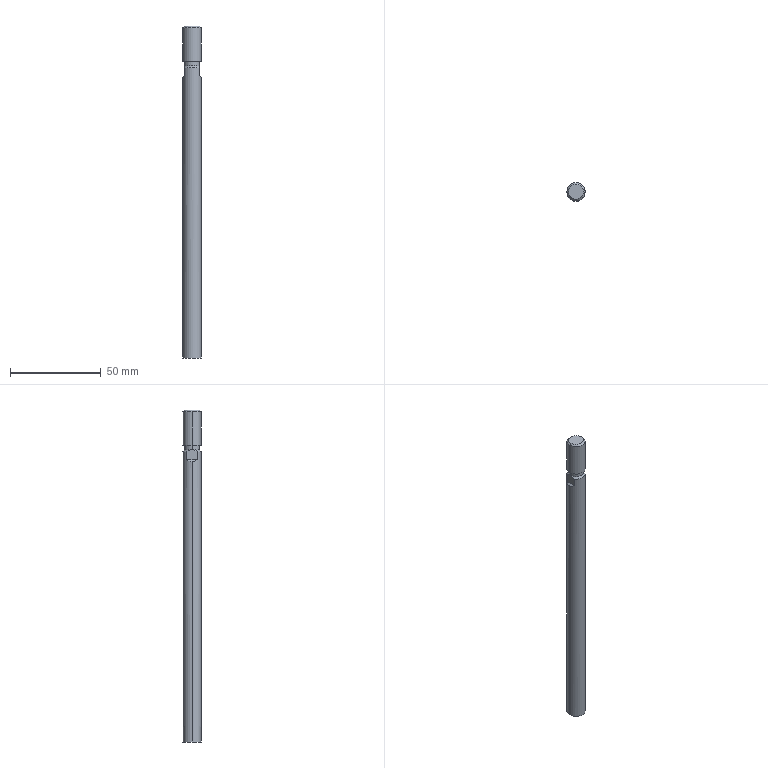Part | STEP file | A_CDM2B25-150-C76(1)_Default | 1 solid | 19 faces | box 10 x 10 x 183 mm | volume 14238 mm3 | cylinder 6 | plane 5 | cone 4 | spline 4 | commonest cylinder face diameters 10 x4 8.16 x2